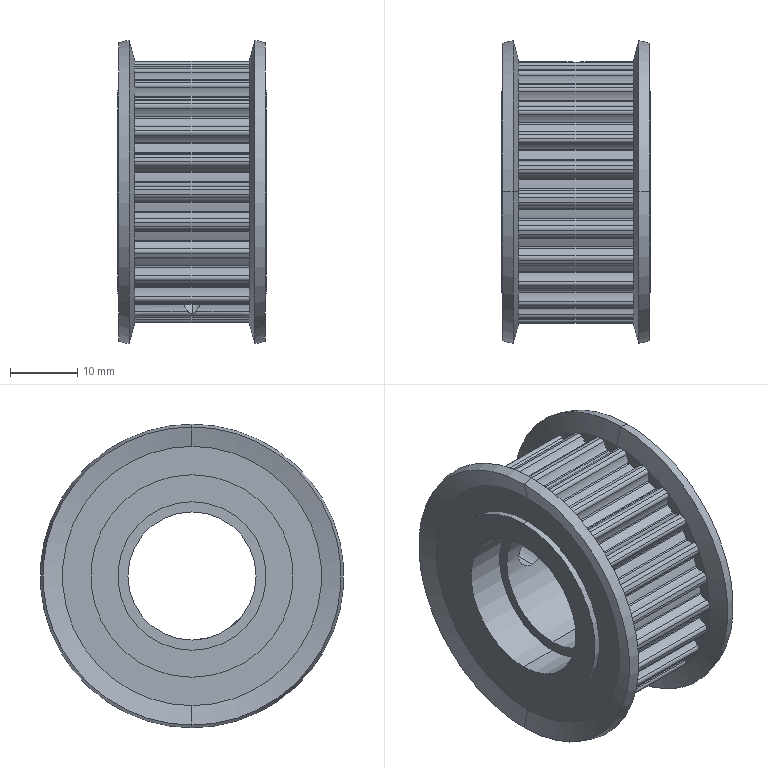Part | SolidWorks | features BaseBody 1 | 1 solid | 294 faces | box 22 x 45 x 45 mm | volume 16795 mm3 | cylinder 226 | plane 56 | cone 12 | commonest cylinder face diameters 0.5 x54 6.55 x54 1.1 x52 35.29 x27 38.83 x25 22 x4